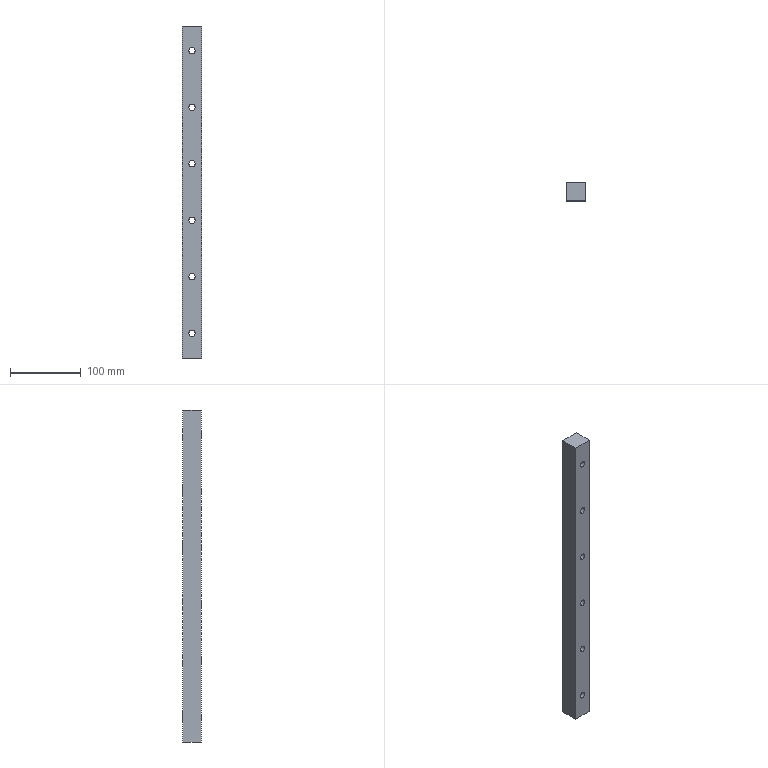Part | SolidWorks | features Extrusion 1, HoleWzd 1, LPattern 1 | 1 solid | 36 faces | box 28 x 26 x 470 mm | volume 326128 mm3 | cylinder 24 | plane 12 | commonest cylinder face diameters 9 x12 15 x12
STEP:
#1=CARTESIAN_POINT('',(0.,-13.,-439.5));
#2=VERTEX_POINT('',#1);
#3=CARTESIAN_POINT('',(0.,-13.,-430.5));
#4=VERTEX_POINT('',#3);
#5=CARTESIAN_POINT('',(0.,-13.,-435.));
#6=DIRECTION('',(0.,1.,0.));
#7=DIRECTION('',(0.,0.,1.));
#8=AXIS2_PLACEMENT_3D('',#5,#6,#7);
#9=CIRCLE('',#8,4.5);
#10=EDGE_CURVE('',#2,#4,#9,.T.);
#11=ORIENTED_EDGE('',*,*,#10,.F.);
#12=CARTESIAN_POINT('',(0.,4.,-439.5));
#13=VERTEX_POINT('',#12);
#14=CARTESIAN_POINT('',(0.,13.,-439.5));
#15=DIRECTION('',(0.,1.,0.));
#16=VECTOR('',#15,1000.);
#17=LINE('',#14,#16);
#18=EDGE_CURVE('',#2,#13,#17,.T.);
#19=ORIENTED_EDGE('',*,*,#18,.T.);
#20=CARTESIAN_POINT('',(0.,4.,-430.5));
#21=VERTEX_POINT('',#20);
#22=CARTESIAN_POINT('',(0.,4.,-435.));
#23=DIRECTION('',(0.,1.,0.));
#24=DIRECTION('',(0.,0.,1.));
#25=AXIS2_PLACEMENT_3D('',#22,#23,#24);
#26=CIRCLE('',#25,4.5);
#27=EDGE_CURVE('',#13,#21,#26,.T.);
#28=ORIENTED_EDGE('',*,*,#27,.T.);
#29=CARTESIAN_POINT('',(0.,13.,-430.5));
#30=DIRECTION('',(0.,1.,0.));
#31=VECTOR('',#30,1000.);
#32=LINE('',#29,#31);
#33=EDGE_CURVE('',#4,#21,#32,.T.);
#34=ORIENTED_EDGE('',*,*,#33,.F.);
#35=EDGE_LOOP('',(#11,#19,#28,#34));
#36=FACE_OUTER_BOUND('',#35,.T.);
#37=CARTESIAN_POINT('',(0.,13.,-435.));
#38=DIRECTION('',(0.,1.,0.));
#39=DIRECTION('',(0.,0.,1.));
#40=AXIS2_PLACEMENT_3D('',#37,#38,#39);
#41=CYLINDRICAL_SURFACE('',#40,4.5);
#42=ADVANCED_FACE('',(#36),#41,.F.);
#43=CARTESIAN_POINT('',(0.,4.,-442.5));
#44=VERTEX_POINT('',#43);
#45=CARTESIAN_POINT('',(0.,4.,-427.5));
#46=VERTEX_POINT('',#45);
#47=CARTESIAN_POINT('',(0.,4.,-435.));
#48=DIRECTION('',(0.,1.,0.));
#49=DIRECTION('',(0.,0.,1.));
#50=AXIS2_PLACEMENT_3D('',#47,#48,#49);
#51=CIRCLE('',#50,7.5);
#52=EDGE_CURVE('',#44,#46,#51,.T.);
#53=ORIENTED_EDGE('',*,*,#52,.F.);
#54=CARTESIAN_POINT('',(0.,13.,-442.5));
#55=VERTEX_POINT('',#54);
#56=CARTESIAN_POINT('',(0.,13.,-442.5));
#57=DIRECTION('',(0.,1.,0.));
#58=VECTOR('',#57,1000.);
#59=LINE('',#56,#58);
#60=EDGE_CURVE('',#44,#55,#59,.T.);
#61=ORIENTED_EDGE('',*,*,#60,.T.);
#62=CARTESIAN_POINT('',(0.,13.,-427.5));
#63=VERTEX_POINT('',#62);
#64=CARTESIAN_POINT('',(0.,13.,-435.));
#65=DIRECTION('',(0.,1.,0.));
#66=DIRECTION('',(0.,0.,1.));
#67=AXIS2_PLACEMENT_3D('',#64,#65,#66);
#68=CIRCLE('',#67,7.5);
#69=EDGE_CURVE('',#55,#63,#68,.T.);
#70=ORIENTED_EDGE('',*,*,#69,.T.);
#71=CARTESIAN_POINT('',(0.,13.,-427.5));
#72=DIRECTION('',(0.,1.,0.));
#73=VECTOR('',#72,1000.);
#74=LINE('',#71,#73);
#75=EDGE_CURVE('',#46,#63,#74,.T.);
#76=ORIENTED_EDGE('',*,*,#75,.F.);
#77=EDGE_LOOP('',(#53,#61,#70,#76));
#78=FACE_OUTER_BOUND('',#77,.T.);
#79=CARTESIAN_POINT('',(0.,13.,-435.));
#80=DIRECTION('',(0.,1.,0.));
#81=DIRECTION('',(0.,0.,1.));
#82=AXIS2_PLACEMENT_3D('',#79,#80,#81);
#83=CYLINDRICAL_SURFACE('',#82,7.5);
#84=ADVANCED_FACE('',(#78),#83,.F.);
#85=CARTESIAN_POINT('',(0.,-13.,-359.5));
#86=VERTEX_POINT('',#85);
#87=CARTESIAN_POINT('',(0.,-13.,-350.5));
#88=VERTEX_POINT('',#87);
#89=CARTESIAN_POINT('',(0.,-13.,-355.));
#90=DIRECTION('',(0.,1.,0.));
#91=DIRECTION('',(0.,0.,1.));
#92=AXIS2_PLACEMENT_3D('',#89,#90,#91);
#93=CIRCLE('',#92,4.5);
#94=EDGE_CURVE('',#86,#88,#93,.T.);
#95=ORIENTED_EDGE('',*,*,#94,.F.);
#96=CARTESIAN_POINT('',(0.,4.,-359.5));
#97=VERTEX_POINT('',#96);
#98=CARTESIAN_POINT('',(0.,13.,-359.5));
#99=DIRECTION('',(0.,1.,0.));
#100=VECTOR('',#99,1000.);
#101=LINE('',#98,#100);
#102=EDGE_CURVE('',#86,#97,#101,.T.);
#103=ORIENTED_EDGE('',*,*,#102,.T.);
#104=CARTESIAN_POINT('',(0.,4.,-350.5));
#105=VERTEX_POINT('',#104);
#106=CARTESIAN_POINT('',(0.,4.,-355.));
#107=DIRECTION('',(0.,1.,0.));
#108=DIRECTION('',(0.,0.,1.));
#109=AXIS2_PLACEMENT_3D('',#106,#107,#108);
#110=CIRCLE('',#109,4.5);
#111=EDGE_CURVE('',#97,#105,#110,.T.);
#112=ORIENTED_EDGE('',*,*,#111,.T.);
#113=CARTESIAN_POINT('',(0.,13.,-350.5));
#114=DIRECTION('',(0.,1.,0.));
#115=VECTOR('',#114,1000.);
#116=LINE('',#113,#115);
#117=EDGE_CURVE('',#88,#105,#116,.T.);
#118=ORIENTED_EDGE('',*,*,#117,.F.);
#119=EDGE_LOOP('',(#95,#103,#112,#118));
#120=FACE_OUTER_BOUND('',#119,.T.);
#121=CARTESIAN_POINT('',(0.,13.,-355.));
#122=DIRECTION('',(0.,1.,0.));
#123=DIRECTION('',(0.,0.,1.));
#124=AXIS2_PLACEMENT_3D('',#121,#122,#123);
#125=CYLINDRICAL_SURFACE('',#124,4.5);
#126=ADVANCED_FACE('',(#120),#125,.F.);
#127=CARTESIAN_POINT('',(0.,4.,-362.5));
#128=VERTEX_POINT('',#127);
#129=CARTESIAN_POINT('',(0.,4.,-347.5));
#130=VERTEX_POINT('',#129);
#131=CARTESIAN_POINT('',(0.,4.,-355.));
#132=DIRECTION('',(0.,1.,0.));
#133=DIRECTION('',(0.,0.,1.));
#134=AXIS2_PLACEMENT_3D('',#131,#132,#133);
#135=CIRCLE('',#134,7.5);
#136=EDGE_CURVE('',#128,#130,#135,.T.);
#137=ORIENTED_EDGE('',*,*,#136,.F.);
#138=CARTESIAN_POINT('',(0.,13.,-362.5));
#139=VERTEX_POINT('',#138);
#140=CARTESIAN_POINT('',(0.,13.,-362.5));
#141=DIRECTION('',(0.,1.,0.));
#142=VECTOR('',#141,1000.);
#143=LINE('',#140,#142);
#144=EDGE_CURVE('',#128,#139,#143,.T.);
#145=ORIENTED_EDGE('',*,*,#144,.T.);
#146=CARTESIAN_POINT('',(0.,13.,-347.5));
#147=VERTEX_POINT('',#146);
#148=CARTESIAN_POINT('',(0.,13.,-355.));
#149=DIRECTION('',(0.,1.,0.));
#150=DIRECTION('',(0.,0.,1.));
#151=AXIS2_PLACEMENT_3D('',#148,#149,#150);
#152=CIRCLE('',#151,7.5);
#153=EDGE_CURVE('',#139,#147,#152,.T.);
#154=ORIENTED_EDGE('',*,*,#153,.T.);
#155=CARTESIAN_POINT('',(0.,13.,-347.5));
#156=DIRECTION('',(0.,1.,0.));
#157=VECTOR('',#156,1000.);
#158=LINE('',#155,#157);
#159=EDGE_CURVE('',#130,#147,#158,.T.);
#160=ORIENTED_EDGE('',*,*,#159,.F.);
#161=EDGE_LOOP('',(#137,#145,#154,#160));
#162=FACE_OUTER_BOUND('',#161,.T.);
#163=CARTESIAN_POINT('',(0.,13.,-355.));
#164=DIRECTION('',(0.,1.,0.));
#165=DIRECTION('',(0.,0.,1.));
#166=AXIS2_PLACEMENT_3D('',#163,#164,#165);
#167=CYLINDRICAL_SURFACE('',#166,7.5);
#168=ADVANCED_FACE('',(#162),#167,.F.);
#169=CARTESIAN_POINT('',(0.,-13.,-279.5));
#170=VERTEX_POINT('',#169);
#171=CARTESIAN_POINT('',(0.,-13.,-270.5));
#172=VERTEX_POINT('',#171);
#173=CARTESIAN_POINT('',(0.,-13.,-275.));
#174=DIRECTION('',(0.,1.,0.));
#175=DIRECTION('',(0.,0.,1.));
#176=AXIS2_PLACEMENT_3D('',#173,#174,#175);
#177=CIRCLE('',#176,4.5);
#178=EDGE_CURVE('',#170,#172,#177,.T.);
#179=ORIENTED_EDGE('',*,*,#178,.F.);
#180=CARTESIAN_POINT('',(0.,4.,-279.5));
#181=VERTEX_POINT('',#180);
#182=CARTESIAN_POINT('',(0.,13.,-279.5));
#183=DIRECTION('',(0.,1.,0.));
#184=VECTOR('',#183,1000.);
#185=LINE('',#182,#184);
#186=EDGE_CURVE('',#170,#181,#185,.T.);
#187=ORIENTED_EDGE('',*,*,#186,.T.);
#188=CARTESIAN_POINT('',(0.,4.,-270.5));
#189=VERTEX_POINT('',#188);
#190=CARTESIAN_POINT('',(0.,4.,-275.));
#191=DIRECTION('',(0.,1.,0.));
#192=DIRECTION('',(0.,0.,1.));
#193=AXIS2_PLACEMENT_3D('',#190,#191,#192);
#194=CIRCLE('',#193,4.5);
#195=EDGE_CURVE('',#181,#189,#194,.T.);
#196=ORIENTED_EDGE('',*,*,#195,.T.);
#197=CARTESIAN_POINT('',(0.,13.,-270.5));
#198=DIRECTION('',(0.,1.,0.));
#199=VECTOR('',#198,1000.);
#200=LINE('',#197,#199);
#201=EDGE_CURVE('',#172,#189,#200,.T.);
#202=ORIENTED_EDGE('',*,*,#201,.F.);
#203=EDGE_LOOP('',(#179,#187,#196,#202));
#204=FACE_OUTER_BOUND('',#203,.T.);
#205=CARTESIAN_POINT('',(0.,13.,-275.));
#206=DIRECTION('',(0.,1.,0.));
#207=DIRECTION('',(0.,0.,1.));
#208=AXIS2_PLACEMENT_3D('',#205,#206,#207);
#209=CYLINDRICAL_SURFACE('',#208,4.5);
#210=ADVANCED_FACE('',(#204),#209,.F.);
#211=CARTESIAN_POINT('',(0.,4.,-282.5));
#212=VERTEX_POINT('',#211);
#213=CARTESIAN_POINT('',(0.,4.,-267.5));
#214=VERTEX_POINT('',#213);
#215=CARTESIAN_POINT('',(0.,4.,-275.));
#216=DIRECTION('',(0.,1.,0.));
#217=DIRECTION('',(0.,0.,1.));
#218=AXIS2_PLACEMENT_3D('',#215,#216,#217);
#219=CIRCLE('',#218,7.5);
#220=EDGE_CURVE('',#212,#214,#219,.T.);
#221=ORIENTED_EDGE('',*,*,#220,.F.);
#222=CARTESIAN_POINT('',(0.,13.,-282.5));
#223=VERTEX_POINT('',#222);
#224=CARTESIAN_POINT('',(0.,13.,-282.5));
#225=DIRECTION('',(0.,1.,0.));
#226=VECTOR('',#225,1000.);
#227=LINE('',#224,#226);
#228=EDGE_CURVE('',#212,#223,#227,.T.);
#229=ORIENTED_EDGE('',*,*,#228,.T.);
#230=CARTESIAN_POINT('',(0.,13.,-267.5));
#231=VERTEX_POINT('',#230);
#232=CARTESIAN_POINT('',(0.,13.,-275.));
#233=DIRECTION('',(0.,1.,0.));
#234=DIRECTION('',(0.,0.,1.));
#235=AXIS2_PLACEMENT_3D('',#232,#233,#234);
#236=CIRCLE('',#235,7.5);
#237=EDGE_CURVE('',#223,#231,#236,.T.);
#238=ORIENTED_EDGE('',*,*,#237,.T.);
#239=CARTESIAN_POINT('',(0.,13.,-267.5));
#240=DIRECTION('',(0.,1.,0.));
#241=VECTOR('',#240,1000.);
#242=LINE('',#239,#241);
#243=EDGE_CURVE('',#214,#231,#242,.T.);
#244=ORIENTED_EDGE('',*,*,#243,.F.);
#245=EDGE_LOOP('',(#221,#229,#238,#244));
#246=FACE_OUTER_BOUND('',#245,.T.);
#247=CARTESIAN_POINT('',(0.,13.,-275.));
#248=DIRECTION('',(0.,1.,0.));
#249=DIRECTION('',(0.,0.,1.));
#250=AXIS2_PLACEMENT_3D('',#247,#248,#249);
#251=CYLINDRICAL_SURFACE('',#250,7.5);
#252=ADVANCED_FACE('',(#246),#251,.F.);
#253=CARTESIAN_POINT('',(0.,-13.,-199.5));
#254=VERTEX_POINT('',#253);
#255=CARTESIAN_POINT('',(0.,-13.,-190.5));
#256=VERTEX_POINT('',#255);
#257=CARTESIAN_POINT('',(0.,-13.,-195.));
#258=DIRECTION('',(0.,1.,0.));
#259=DIRECTION('',(0.,0.,1.));
#260=AXIS2_PLACEMENT_3D('',#257,#258,#259);
#261=CIRCLE('',#260,4.5);
#262=EDGE_CURVE('',#254,#256,#261,.T.);
#263=ORIENTED_EDGE('',*,*,#262,.F.);
#264=CARTESIAN_POINT('',(0.,4.,-199.5));
#265=VERTEX_POINT('',#264);
#266=CARTESIAN_POINT('',(0.,13.,-199.5));
#267=DIRECTION('',(0.,1.,0.));
#268=VECTOR('',#267,1000.);
#269=LINE('',#266,#268);
#270=EDGE_CURVE('',#254,#265,#269,.T.);
#271=ORIENTED_EDGE('',*,*,#270,.T.);
#272=CARTESIAN_POINT('',(0.,4.,-190.5));
#273=VERTEX_POINT('',#272);
#274=CARTESIAN_POINT('',(0.,4.,-195.));
#275=DIRECTION('',(0.,1.,0.));
#276=DIRECTION('',(0.,0.,1.));
#277=AXIS2_PLACEMENT_3D('',#274,#275,#276);
#278=CIRCLE('',#277,4.5);
#279=EDGE_CURVE('',#265,#273,#278,.T.);
#280=ORIENTED_EDGE('',*,*,#279,.T.);
#281=CARTESIAN_POINT('',(0.,13.,-190.5));
#282=DIRECTION('',(0.,1.,0.));
#283=VECTOR('',#282,1000.);
#284=LINE('',#281,#283);
#285=EDGE_CURVE('',#256,#273,#284,.T.);
#286=ORIENTED_EDGE('',*,*,#285,.F.);
#287=EDGE_LOOP('',(#263,#271,#280,#286));
#288=FACE_OUTER_BOUND('',#287,.T.);
#289=CARTESIAN_POINT('',(0.,13.,-195.));
#290=DIRECTION('',(0.,1.,0.));
#291=DIRECTION('',(0.,0.,1.));
#292=AXIS2_PLACEMENT_3D('',#289,#290,#291);
#293=CYLINDRICAL_SURFACE('',#292,4.5);
#294=ADVANCED_FACE('',(#288),#293,.F.);
#295=CARTESIAN_POINT('',(0.,4.,-202.5));
#296=VERTEX_POINT('',#295);
#297=CARTESIAN_POINT('',(0.,4.,-187.5));
#298=VERTEX_POINT('',#297);
#299=CARTESIAN_POINT('',(0.,4.,-195.));
#300=DIRECTION('',(0.,1.,0.));
#301=DIRECTION('',(0.,0.,1.));
#302=AXIS2_PLACEMENT_3D('',#299,#300,#301);
#303=CIRCLE('',#302,7.5);
#304=EDGE_CURVE('',#296,#298,#303,.T.);
#305=ORIENTED_EDGE('',*,*,#304,.F.);
#306=CARTESIAN_POINT('',(0.,13.,-202.5));
#307=VERTEX_POINT('',#306);
#308=CARTESIAN_POINT('',(0.,13.,-202.5));
#309=DIRECTION('',(0.,1.,0.));
#310=VECTOR('',#309,1000.);
#311=LINE('',#308,#310);
#312=EDGE_CURVE('',#296,#307,#311,.T.);
#313=ORIENTED_EDGE('',*,*,#312,.T.);
#314=CARTESIAN_POINT('',(0.,13.,-187.5));
#315=VERTEX_POINT('',#314);
#316=CARTESIAN_POINT('',(0.,13.,-195.));
#317=DIRECTION('',(0.,1.,0.));
#318=DIRECTION('',(0.,0.,1.));
#319=AXIS2_PLACEMENT_3D('',#316,#317,#318);
#320=CIRCLE('',#319,7.5);
#321=EDGE_CURVE('',#307,#315,#320,.T.);
#322=ORIENTED_EDGE('',*,*,#321,.T.);
#323=CARTESIAN_POINT('',(0.,13.,-187.5));
#324=DIRECTION('',(0.,1.,0.));
#325=VECTOR('',#324,1000.);
#326=LINE('',#323,#325);
#327=EDGE_CURVE('',#298,#315,#326,.T.);
#328=ORIENTED_EDGE('',*,*,#327,.F.);
#329=EDGE_LOOP('',(#305,#313,#322,#328));
#330=FACE_OUTER_BOUND('',#329,.T.);
#331=CARTESIAN_POINT('',(0.,13.,-195.));
#332=DIRECTION('',(0.,1.,0.));
#333=DIRECTION('',(0.,0.,1.));
#334=AXIS2_PLACEMENT_3D('',#331,#332,#333);
#335=CYLINDRICAL_SURFACE('',#334,7.5);
#336=ADVANCED_FACE('',(#330),#335,.F.);
#337=CARTESIAN_POINT('',(0.,4.,-122.5));
#338=VERTEX_POINT('',#337);
#339=CARTESIAN_POINT('',(0.,4.,-107.5));
#340=VERTEX_POINT('',#339);
#341=CARTESIAN_POINT('',(0.,4.,-115.));
#342=DIRECTION('',(0.,1.,0.));
#343=DIRECTION('',(0.,0.,1.));
#344=AXIS2_PLACEMENT_3D('',#341,#342,#343);
#345=CIRCLE('',#344,7.5);
#346=EDGE_CURVE('',#338,#340,#345,.T.);
#347=ORIENTED_EDGE('',*,*,#346,.F.);
#348=CARTESIAN_POINT('',(0.,13.,-122.5));
#349=VERTEX_POINT('',#348);
#350=CARTESIAN_POINT('',(0.,13.,-122.5));
#351=DIRECTION('',(0.,1.,0.));
#352=VECTOR('',#351,1000.);
#353=LINE('',#350,#352);
#354=EDGE_CURVE('',#338,#349,#353,.T.);
#355=ORIENTED_EDGE('',*,*,#354,.T.);
#356=CARTESIAN_POINT('',(0.,13.,-107.5));
#357=VERTEX_POINT('',#356);
#358=CARTESIAN_POINT('',(0.,13.,-115.));
#359=DIRECTION('',(0.,1.,0.));
#360=DIRECTION('',(0.,0.,1.));
#361=AXIS2_PLACEMENT_3D('',#358,#359,#360);
#362=CIRCLE('',#361,7.5);
#363=EDGE_CURVE('',#349,#357,#362,.T.);
#364=ORIENTED_EDGE('',*,*,#363,.T.);
#365=CARTESIAN_POINT('',(0.,13.,-107.5));
#366=DIRECTION('',(0.,1.,0.));
#367=VECTOR('',#366,1000.);
#368=LINE('',#365,#367);
#369=EDGE_CURVE('',#340,#357,#368,.T.);
#370=ORIENTED_EDGE('',*,*,#369,.F.);
#371=EDGE_LOOP('',(#347,#355,#364,#370));
#372=FACE_OUTER_BOUND('',#371,.T.);
#373=CARTESIAN_POINT('',(0.,13.,-115.));
#374=DIRECTION('',(0.,1.,0.));
#375=DIRECTION('',(0.,0.,1.));
#376=AXIS2_PLACEMENT_3D('',#373,#374,#375);
#377=CYLINDRICAL_SURFACE('',#376,7.5);
#378=ADVANCED_FACE('',(#372),#377,.F.);
#379=CARTESIAN_POINT('',(0.,-13.,-119.5));
#380=VERTEX_POINT('',#379);
#381=CARTESIAN_POINT('',(0.,-13.,-110.5));
#382=VERTEX_POINT('',#381);
#383=CARTESIAN_POINT('',(0.,-13.,-115.));
#384=DIRECTION('',(0.,1.,0.));
#385=DIRECTION('',(0.,0.,1.));
#386=AXIS2_PLACEMENT_3D('',#383,#384,#385);
#387=CIRCLE('',#386,4.5);
#388=EDGE_CURVE('',#380,#382,#387,.T.);
#389=ORIENTED_EDGE('',*,*,#388,.F.);
#390=CARTESIAN_POINT('',(0.,4.,-119.5));
#391=VERTEX_POINT('',#390);
#392=CARTESIAN_POINT('',(0.,13.,-119.5));
#393=DIRECTION('',(0.,1.,0.));
#394=VECTOR('',#393,1000.);
#395=LINE('',#392,#394);
#396=EDGE_CURVE('',#380,#391,#395,.T.);
#397=ORIENTED_EDGE('',*,*,#396,.T.);
#398=CARTESIAN_POINT('',(0.,4.,-110.5));
#399=VERTEX_POINT('',#398);
#400=CARTESIAN_POINT('',(0.,4.,-115.));
#401=DIRECTION('',(0.,1.,0.));
#402=DIRECTION('',(0.,0.,1.));
#403=AXIS2_PLACEMENT_3D('',#400,#401,#402);
#404=CIRCLE('',#403,4.5);
#405=EDGE_CURVE('',#391,#399,#404,.T.);
#406=ORIENTED_EDGE('',*,*,#405,.T.);
#407=CARTESIAN_POINT('',(0.,13.,-110.5));
#408=DIRECTION('',(0.,1.,0.));
#409=VECTOR('',#408,1000.);
#410=LINE('',#407,#409);
#411=EDGE_CURVE('',#382,#399,#410,.T.);
#412=ORIENTED_EDGE('',*,*,#411,.F.);
#413=EDGE_LOOP('',(#389,#397,#406,#412));
#414=FACE_OUTER_BOUND('',#413,.T.);
#415=CARTESIAN_POINT('',(0.,13.,-115.));
#416=DIRECTION('',(0.,1.,0.));
#417=DIRECTION('',(0.,0.,1.));
#418=AXIS2_PLACEMENT_3D('',#415,#416,#417);
#419=CYLINDRICAL_SURFACE('',#418,4.5);
#420=ADVANCED_FACE('',(#414),#419,.F.);
#421=CARTESIAN_POINT('',(0.,4.,-42.5));
#422=VERTEX_POINT('',#421);
#423=CARTESIAN_POINT('',(0.,4.,-27.5));
#424=VERTEX_POINT('',#423);
#425=CARTESIAN_POINT('',(0.,4.,-35.));
#426=DIRECTION('',(0.,1.,0.));
#427=DIRECTION('',(0.,0.,1.));
#428=AXIS2_PLACEMENT_3D('',#425,#426,#427);
#429=CIRCLE('',#428,7.5);
#430=EDGE_CURVE('',#422,#424,#429,.T.);
#431=ORIENTED_EDGE('',*,*,#430,.F.);
#432=CARTESIAN_POINT('',(0.,13.,-42.5));
#433=VERTEX_POINT('',#432);
#434=CARTESIAN_POINT('',(0.,13.,-42.5));
#435=DIRECTION('',(0.,1.,0.));
#436=VECTOR('',#435,1000.);
#437=LINE('',#434,#436);
#438=EDGE_CURVE('',#422,#433,#437,.T.);
#439=ORIENTED_EDGE('',*,*,#438,.T.);
#440=CARTESIAN_POINT('',(0.,13.,-27.5));
#441=VERTEX_POINT('',#440);
#442=CARTESIAN_POINT('',(0.,13.,-35.));
#443=DIRECTION('',(0.,1.,0.));
#444=DIRECTION('',(0.,0.,1.));
#445=AXIS2_PLACEMENT_3D('',#442,#443,#444);
#446=CIRCLE('',#445,7.5);
#447=EDGE_CURVE('',#433,#441,#446,.T.);
#448=ORIENTED_EDGE('',*,*,#447,.T.);
#449=CARTESIAN_POINT('',(0.,13.,-27.5));
#450=DIRECTION('',(0.,1.,0.));
#451=VECTOR('',#450,1000.);
#452=LINE('',#449,#451);
#453=EDGE_CURVE('',#424,#441,#452,.T.);
#454=ORIENTED_EDGE('',*,*,#453,.F.);
#455=EDGE_LOOP('',(#431,#439,#448,#454));
#456=FACE_OUTER_BOUND('',#455,.T.);
#457=CARTESIAN_POINT('',(0.,13.,-35.));
#458=DIRECTION('',(0.,1.,0.));
#459=DIRECTION('',(0.,0.,1.));
#460=AXIS2_PLACEMENT_3D('',#457,#458,#459);
#461=CYLINDRICAL_SURFACE('',#460,7.5);
#462=ADVANCED_FACE('',(#456),#461,.F.);
#463=CARTESIAN_POINT('',(0.,-13.,-39.5));
#464=VERTEX_POINT('',#463);
#465=CARTESIAN_POINT('',(0.,-13.,-30.5));
#466=VERTEX_POINT('',#465);
#467=CARTESIAN_POINT('',(0.,-13.,-35.));
#468=DIRECTION('',(0.,1.,0.));
#469=DIRECTION('',(0.,0.,1.));
#470=AXIS2_PLACEMENT_3D('',#467,#468,#469);
#471=CIRCLE('',#470,4.5);
#472=EDGE_CURVE('',#464,#466,#471,.T.);
#473=ORIENTED_EDGE('',*,*,#472,.F.);
#474=CARTESIAN_POINT('',(0.,4.,-39.5));
#475=VERTEX_POINT('',#474);
#476=CARTESIAN_POINT('',(0.,13.,-39.5));
#477=DIRECTION('',(0.,1.,0.));
#478=VECTOR('',#477,1000.);
#479=LINE('',#476,#478);
#480=EDGE_CURVE('',#464,#475,#479,.T.);
#481=ORIENTED_EDGE('',*,*,#480,.T.);
#482=CARTESIAN_POINT('',(0.,4.,-30.5));
#483=VERTEX_POINT('',#482);
#484=CARTESIAN_POINT('',(0.,4.,-35.));
#485=DIRECTION('',(0.,1.,0.));
#486=DIRECTION('',(0.,0.,1.));
#487=AXIS2_PLACEMENT_3D('',#484,#485,#486);
#488=CIRCLE('',#487,4.5);
#489=EDGE_CURVE('',#475,#483,#488,.T.);
#490=ORIENTED_EDGE('',*,*,#489,.T.);
#491=CARTESIAN_POINT('',(0.,13.,-30.5));
#492=DIRECTION('',(0.,1.,0.));
#493=VECTOR('',#492,1000.);
#494=LINE('',#491,#493);
#495=EDGE_CURVE('',#466,#483,#494,.T.);
#496=ORIENTED_EDGE('',*,*,#495,.F.);
#497=EDGE_LOOP('',(#473,#481,#490,#496));
#498=FACE_OUTER_BOUND('',#497,.T.);
#499=CARTESIAN_POINT('',(0.,13.,-35.));
#500=DIRECTION('',(0.,1.,0.));
#501=DIRECTION('',(0.,0.,1.));
#502=AXIS2_PLACEMENT_3D('',#499,#500,#501);
#503=CYLINDRICAL_SURFACE('',#502,4.5);
#504=ADVANCED_FACE('',(#498),#503,.F.);
#505=CARTESIAN_POINT('',(14.,-13.,0.));
#506=VERTEX_POINT('',#505);
#507=CARTESIAN_POINT('',(14.,13.,0.));
#508=VERTEX_POINT('',#507);
#509=CARTESIAN_POINT('',(14.,13.,0.));
#510=DIRECTION('',(0.,1.,0.));
#511=VECTOR('',#510,1000.);
#512=LINE('',#509,#511);
#513=EDGE_CURVE('',#506,#508,#512,.T.);
#514=ORIENTED_EDGE('',*,*,#513,.F.);
#515=CARTESIAN_POINT('',(14.,-13.,-470.));
#516=VERTEX_POINT('',#515);
#517=CARTESIAN_POINT('',(14.,-13.,-470.));
#518=DIRECTION('',(0.,0.,1.));
#519=VECTOR('',#518,1000.);
#520=LINE('',#517,#519);
#521=EDGE_CURVE('',#516,#506,#520,.T.);
#522=ORIENTED_EDGE('',*,*,#521,.F.);
#523=CARTESIAN_POINT('',(14.,13.,-470.));
#524=VERTEX_POINT('',#523);
#525=CARTESIAN_POINT('',(14.,13.,-470.));
#526=DIRECTION('',(0.,1.,0.));
#527=VECTOR('',#526,1000.);
#528=LINE('',#525,#527);
#529=EDGE_CURVE('',#516,#524,#528,.T.);
#530=ORIENTED_EDGE('',*,*,#529,.T.);
#531=CARTESIAN_POINT('',(14.,13.,-470.));
#532=DIRECTION('',(0.,0.,1.));
#533=VECTOR('',#532,1000.);
#534=LINE('',#531,#533);
#535=EDGE_CURVE('',#524,#508,#534,.T.);
#536=ORIENTED_EDGE('',*,*,#535,.T.);
#537=EDGE_LOOP('',(#514,#522,#530,#536));
#538=FACE_OUTER_BOUND('',#537,.T.);
#539=CARTESIAN_POINT('',(14.,13.,-470.));
#540=DIRECTION('',(1.,0.,0.));
#541=DIRECTION('',(0.,1.,0.));
#542=AXIS2_PLACEMENT_3D('',#539,#540,#541);
#543=PLANE('',#542);
#544=ADVANCED_FACE('',(#538),#543,.T.);
#545=CARTESIAN_POINT('',(0.,-13.,-115.));
#546=DIRECTION('',(0.,1.,0.));
#547=DIRECTION('',(0.,0.,1.));
#548=AXIS2_PLACEMENT_3D('',#545,#546,#547);
#549=CIRCLE('',#548,4.5);
#550=EDGE_CURVE('',#382,#380,#549,.T.);
#551=ORIENTED_EDGE('',*,*,#550,.T.);
#552=ORIENTED_EDGE('',*,*,#388,.T.);
#553=EDGE_LOOP('',(#551,#552));
#554=FACE_BOUND('',#553,.T.);
#555=CARTESIAN_POINT('',(0.,-13.,-35.));
#556=DIRECTION('',(0.,1.,0.));
#557=DIRECTION('',(0.,0.,1.));
#558=AXIS2_PLACEMENT_3D('',#555,#556,#557);
#559=CIRCLE('',#558,4.5);
#560=EDGE_CURVE('',#466,#464,#559,.T.);
#561=ORIENTED_EDGE('',*,*,#560,.T.);
#562=ORIENTED_EDGE('',*,*,#472,.T.);
#563=EDGE_LOOP('',(#561,#562));
#564=FACE_BOUND('',#563,.T.);
#565=CARTESIAN_POINT('',(-14.,-13.,0.));
#566=VERTEX_POINT('',#565);
#567=CARTESIAN_POINT('',(-14.,-13.,0.));
#568=DIRECTION('',(1.,0.,0.));
#569=VECTOR('',#568,1000.);
#570=LINE('',#567,#569);
#571=EDGE_CURVE('',#566,#506,#570,.T.);
#572=ORIENTED_EDGE('',*,*,#571,.F.);
#573=CARTESIAN_POINT('',(-14.,-13.,-470.));
#574=VERTEX_POINT('',#573);
#575=CARTESIAN_POINT('',(-14.,-13.,-470.));
#576=DIRECTION('',(0.,0.,1.));
#577=VECTOR('',#576,1000.);
#578=LINE('',#575,#577);
#579=EDGE_CURVE('',#574,#566,#578,.T.);
#580=ORIENTED_EDGE('',*,*,#579,.F.);
#581=CARTESIAN_POINT('',(-14.,-13.,-470.));
#582=DIRECTION('',(1.,0.,0.));
#583=VECTOR('',#582,1000.);
#584=LINE('',#581,#583);
#585=EDGE_CURVE('',#574,#516,#584,.T.);
#586=ORIENTED_EDGE('',*,*,#585,.T.);
#587=ORIENTED_EDGE('',*,*,#521,.T.);
#588=EDGE_LOOP('',(#572,#580,#586,#587));
#589=FACE_OUTER_BOUND('',#588,.T.);
#590=CARTESIAN_POINT('',(0.,-13.,-195.));
#591=DIRECTION('',(0.,1.,0.));
#592=DIRECTION('',(0.,0.,1.));
#593=AXIS2_PLACEMENT_3D('',#590,#591,#592);
#594=CIRCLE('',#593,4.5);
#595=EDGE_CURVE('',#256,#254,#594,.T.);
#596=ORIENTED_EDGE('',*,*,#595,.T.);
#597=ORIENTED_EDGE('',*,*,#262,.T.);
#598=EDGE_LOOP('',(#596,#597));
#599=FACE_BOUND('',#598,.T.);
#600=CARTESIAN_POINT('',(0.,-13.,-275.));
#601=DIRECTION('',(0.,1.,0.));
#602=DIRECTION('',(0.,0.,1.));
#603=AXIS2_PLACEMENT_3D('',#600,#601,#602);
#604=CIRCLE('',#603,4.5);
#605=EDGE_CURVE('',#172,#170,#604,.T.);
#606=ORIENTED_EDGE('',*,*,#605,.T.);
#607=ORIENTED_EDGE('',*,*,#178,.T.);
#608=EDGE_LOOP('',(#606,#607));
#609=FACE_BOUND('',#608,.T.);
#610=CARTESIAN_POINT('',(0.,-13.,-355.));
#611=DIRECTION('',(0.,1.,0.));
#612=DIRECTION('',(0.,0.,1.));
#613=AXIS2_PLACEMENT_3D('',#610,#611,#612);
#614=CIRCLE('',#613,4.5);
#615=EDGE_CURVE('',#88,#86,#614,.T.);
#616=ORIENTED_EDGE('',*,*,#615,.T.);
#617=ORIENTED_EDGE('',*,*,#94,.T.);
#618=EDGE_LOOP('',(#616,#617));
#619=FACE_BOUND('',#618,.T.);
#620=CARTESIAN_POINT('',(0.,-13.,-435.));
#621=DIRECTION('',(0.,1.,0.));
#622=DIRECTION('',(0.,0.,1.));
#623=AXIS2_PLACEMENT_3D('',#620,#621,#622);
#624=CIRCLE('',#623,4.5);
#625=EDGE_CURVE('',#4,#2,#624,.T.);
#626=ORIENTED_EDGE('',*,*,#625,.T.);
#627=ORIENTED_EDGE('',*,*,#10,.T.);
#628=EDGE_LOOP('',(#626,#627));
#629=FACE_BOUND('',#628,.T.);
#630=CARTESIAN_POINT('',(-14.,-13.,-470.));
#631=DIRECTION('',(0.,-1.,0.));
#632=DIRECTION('',(0.,0.,-1.));
#633=AXIS2_PLACEMENT_3D('',#630,#631,#632);
#634=PLANE('',#633);
#635=ADVANCED_FACE('',(#554,#564,#589,#599,#609,#619,#629),#634,.T.);
#636=CARTESIAN_POINT('',(-14.,13.,0.));
#637=VERTEX_POINT('',#636);
#638=CARTESIAN_POINT('',(-14.,13.,0.));
#639=DIRECTION('',(0.,-1.,0.));
#640=VECTOR('',#639,1000.);
#641=LINE('',#638,#640);
#642=EDGE_CURVE('',#637,#566,#641,.T.);
#643=ORIENTED_EDGE('',*,*,#642,.F.);
#644=CARTESIAN_POINT('',(-14.,13.,-470.));
#645=VERTEX_POINT('',#644);
#646=CARTESIAN_POINT('',(-14.,13.,-470.));
#647=DIRECTION('',(0.,0.,1.));
#648=VECTOR('',#647,1000.);
#649=LINE('',#646,#648);
#650=EDGE_CURVE('',#645,#637,#649,.T.);
#651=ORIENTED_EDGE('',*,*,#650,.F.);
#652=CARTESIAN_POINT('',(-14.,13.,-470.));
#653=DIRECTION('',(0.,-1.,0.));
#654=VECTOR('',#653,1000.);
#655=LINE('',#652,#654);
#656=EDGE_CURVE('',#645,#574,#655,.T.);
#657=ORIENTED_EDGE('',*,*,#656,.T.);
#658=ORIENTED_EDGE('',*,*,#579,.T.);
#659=EDGE_LOOP('',(#643,#651,#657,#658));
#660=FACE_OUTER_BOUND('',#659,.T.);
#661=CARTESIAN_POINT('',(-14.,13.,-470.));
#662=DIRECTION('',(-1.,0.,0.));
#663=DIRECTION('',(0.,-1.,0.));
#664=AXIS2_PLACEMENT_3D('',#661,#662,#663);
#665=PLANE('',#664);
#666=ADVANCED_FACE('',(#660),#665,.T.);
#667=CARTESIAN_POINT('',(0.,13.,-115.));
#668=DIRECTION('',(0.,1.,0.));
#669=DIRECTION('',(0.,0.,1.));
#670=AXIS2_PLACEMENT_3D('',#667,#668,#669);
#671=CIRCLE('',#670,7.5);
#672=EDGE_CURVE('',#357,#349,#671,.T.);
#673=ORIENTED_EDGE('',*,*,#672,.F.);
#674=ORIENTED_EDGE('',*,*,#363,.F.);
#675=EDGE_LOOP('',(#673,#674));
#676=FACE_BOUND('',#675,.T.);
#677=CARTESIAN_POINT('',(0.,13.,-35.));
#678=DIRECTION('',(0.,1.,0.));
#679=DIRECTION('',(0.,0.,1.));
#680=AXIS2_PLACEMENT_3D('',#677,#678,#679);
#681=CIRCLE('',#680,7.5);
#682=EDGE_CURVE('',#441,#433,#681,.T.);
#683=ORIENTED_EDGE('',*,*,#682,.F.);
#684=ORIENTED_EDGE('',*,*,#447,.F.);
#685=EDGE_LOOP('',(#683,#684));
#686=FACE_BOUND('',#685,.T.);
#687=CARTESIAN_POINT('',(-14.,13.,0.));
#688=DIRECTION('',(-1.,0.,0.));
#689=VECTOR('',#688,1000.);
#690=LINE('',#687,#689);
#691=EDGE_CURVE('',#508,#637,#690,.T.);
#692=ORIENTED_EDGE('',*,*,#691,.F.);
#693=ORIENTED_EDGE('',*,*,#535,.F.);
#694=CARTESIAN_POINT('',(-14.,13.,-470.));
#695=DIRECTION('',(-1.,0.,0.));
#696=VECTOR('',#695,1000.);
#697=LINE('',#694,#696);
#698=EDGE_CURVE('',#524,#645,#697,.T.);
#699=ORIENTED_EDGE('',*,*,#698,.T.);
#700=ORIENTED_EDGE('',*,*,#650,.T.);
#701=EDGE_LOOP('',(#692,#693,#699,#700));
#702=FACE_OUTER_BOUND('',#701,.T.);
#703=CARTESIAN_POINT('',(0.,13.,-195.));
#704=DIRECTION('',(0.,1.,0.));
#705=DIRECTION('',(0.,0.,1.));
#706=AXIS2_PLACEMENT_3D('',#703,#704,#705);
#707=CIRCLE('',#706,7.5);
#708=EDGE_CURVE('',#315,#307,#707,.T.);
#709=ORIENTED_EDGE('',*,*,#708,.F.);
#710=ORIENTED_EDGE('',*,*,#321,.F.);
#711=EDGE_LOOP('',(#709,#710));
#712=FACE_BOUND('',#711,.T.);
#713=CARTESIAN_POINT('',(0.,13.,-275.));
#714=DIRECTION('',(0.,1.,0.));
#715=DIRECTION('',(0.,0.,1.));
#716=AXIS2_PLACEMENT_3D('',#713,#714,#715);
#717=CIRCLE('',#716,7.5);
#718=EDGE_CURVE('',#231,#223,#717,.T.);
#719=ORIENTED_EDGE('',*,*,#718,.F.);
#720=ORIENTED_EDGE('',*,*,#237,.F.);
#721=EDGE_LOOP('',(#719,#720));
#722=FACE_BOUND('',#721,.T.);
#723=CARTESIAN_POINT('',(0.,13.,-355.));
#724=DIRECTION('',(0.,1.,0.));
#725=DIRECTION('',(0.,0.,1.));
#726=AXIS2_PLACEMENT_3D('',#723,#724,#725);
#727=CIRCLE('',#726,7.5);
#728=EDGE_CURVE('',#147,#139,#727,.T.);
#729=ORIENTED_EDGE('',*,*,#728,.F.);
#730=ORIENTED_EDGE('',*,*,#153,.F.);
#731=EDGE_LOOP('',(#729,#730));
#732=FACE_BOUND('',#731,.T.);
#733=CARTESIAN_POINT('',(0.,13.,-435.));
#734=DIRECTION('',(0.,1.,0.));
#735=DIRECTION('',(0.,0.,1.));
#736=AXIS2_PLACEMENT_3D('',#733,#734,#735);
#737=CIRCLE('',#736,7.5);
#738=EDGE_CURVE('',#63,#55,#737,.T.);
#739=ORIENTED_EDGE('',*,*,#738,.F.);
#740=ORIENTED_EDGE('',*,*,#69,.F.);
#741=EDGE_LOOP('',(#739,#740));
#742=FACE_BOUND('',#741,.T.);
#743=CARTESIAN_POINT('',(-14.,13.,-470.));
#744=DIRECTION('',(0.,1.,0.));
#745=DIRECTION('',(0.,0.,1.));
#746=AXIS2_PLACEMENT_3D('',#743,#744,#745);
#747=PLANE('',#746);
#748=ADVANCED_FACE('',(#676,#686,#702,#712,#722,#732,#742),#747,.T.);
#749=ORIENTED_EDGE('',*,*,#529,.F.);
#750=ORIENTED_EDGE('',*,*,#585,.F.);
#751=ORIENTED_EDGE('',*,*,#656,.F.);
#752=ORIENTED_EDGE('',*,*,#698,.F.);
#753=EDGE_LOOP('',(#749,#750,#751,#752));
#754=FACE_OUTER_BOUND('',#753,.T.);
#755=CARTESIAN_POINT('',(14.,-13.,-470.));
#756=DIRECTION('',(0.,0.,1.));
#757=DIRECTION('',(1.,0.,0.));
#758=AXIS2_PLACEMENT_3D('',#755,#756,#757);
#759=PLANE('',#758);
#760=ADVANCED_FACE('',(#754),#759,.F.);
#761=ORIENTED_EDGE('',*,*,#513,.T.);
#762=ORIENTED_EDGE('',*,*,#691,.T.);
#763=ORIENTED_EDGE('',*,*,#642,.T.);
#764=ORIENTED_EDGE('',*,*,#571,.T.);
#765=EDGE_LOOP('',(#761,#762,#763,#764));
#766=FACE_OUTER_BOUND('',#765,.T.);
#767=CARTESIAN_POINT('',(14.,-13.,0.));
#768=DIRECTION('',(0.,0.,1.));
#769=DIRECTION('',(1.,0.,0.));
#770=AXIS2_PLACEMENT_3D('',#767,#768,#769);
#771=PLANE('',#770);
#772=ADVANCED_FACE('',(#766),#771,.T.);
#773=ORIENTED_EDGE('',*,*,#480,.F.);
#774=ORIENTED_EDGE('',*,*,#560,.F.);
#775=ORIENTED_EDGE('',*,*,#495,.T.);
#776=CARTESIAN_POINT('',(0.,4.,-35.));
#777=DIRECTION('',(0.,1.,0.));
#778=DIRECTION('',(0.,0.,1.));
#779=AXIS2_PLACEMENT_3D('',#776,#777,#778);
#780=CIRCLE('',#779,4.5);
#781=EDGE_CURVE('',#483,#475,#780,.T.);
#782=ORIENTED_EDGE('',*,*,#781,.T.);
#783=EDGE_LOOP('',(#773,#774,#775,#782));
#784=FACE_OUTER_BOUND('',#783,.T.);
#785=CARTESIAN_POINT('',(0.,13.,-35.));
#786=DIRECTION('',(0.,1.,0.));
#787=DIRECTION('',(0.,0.,1.));
#788=AXIS2_PLACEMENT_3D('',#785,#786,#787);
#789=CYLINDRICAL_SURFACE('',#788,4.5);
#790=ADVANCED_FACE('',(#784),#789,.F.);
#791=ORIENTED_EDGE('',*,*,#781,.F.);
#792=ORIENTED_EDGE('',*,*,#489,.F.);
#793=EDGE_LOOP('',(#791,#792));
#794=FACE_BOUND('',#793,.T.);
#795=CARTESIAN_POINT('',(0.,4.,-35.));
#796=DIRECTION('',(0.,1.,0.));
#797=DIRECTION('',(0.,0.,1.));
#798=AXIS2_PLACEMENT_3D('',#795,#796,#797);
#799=CIRCLE('',#798,7.5);
#800=EDGE_CURVE('',#424,#422,#799,.T.);
#801=ORIENTED_EDGE('',*,*,#800,.T.);
#802=ORIENTED_EDGE('',*,*,#430,.T.);
#803=EDGE_LOOP('',(#801,#802));
#804=FACE_OUTER_BOUND('',#803,.T.);
#805=CARTESIAN_POINT('',(4.5,4.,-35.));
#806=DIRECTION('',(0.,-1.,0.));
#807=DIRECTION('',(0.,0.,-1.));
#808=AXIS2_PLACEMENT_3D('',#805,#806,#807);
#809=PLANE('',#808);
#810=ADVANCED_FACE('',(#794,#804),#809,.F.);
#811=ORIENTED_EDGE('',*,*,#438,.F.);
#812=ORIENTED_EDGE('',*,*,#800,.F.);
#813=ORIENTED_EDGE('',*,*,#453,.T.);
#814=ORIENTED_EDGE('',*,*,#682,.T.);
#815=EDGE_LOOP('',(#811,#812,#813,#814));
#816=FACE_OUTER_BOUND('',#815,.T.);
#817=CARTESIAN_POINT('',(0.,13.,-35.));
#818=DIRECTION('',(0.,1.,0.));
#819=DIRECTION('',(0.,0.,1.));
#820=AXIS2_PLACEMENT_3D('',#817,#818,#819);
#821=CYLINDRICAL_SURFACE('',#820,7.5);
#822=ADVANCED_FACE('',(#816),#821,.F.);
#823=ORIENTED_EDGE('',*,*,#396,.F.);
#824=ORIENTED_EDGE('',*,*,#550,.F.);
#825=ORIENTED_EDGE('',*,*,#411,.T.);
#826=CARTESIAN_POINT('',(0.,4.,-115.));
#827=DIRECTION('',(0.,1.,0.));
#828=DIRECTION('',(0.,0.,1.));
#829=AXIS2_PLACEMENT_3D('',#826,#827,#828);
#830=CIRCLE('',#829,4.5);
#831=EDGE_CURVE('',#399,#391,#830,.T.);
#832=ORIENTED_EDGE('',*,*,#831,.T.);
#833=EDGE_LOOP('',(#823,#824,#825,#832));
#834=FACE_OUTER_BOUND('',#833,.T.);
#835=CARTESIAN_POINT('',(0.,13.,-115.));
#836=DIRECTION('',(0.,1.,0.));
#837=DIRECTION('',(0.,0.,1.));
#838=AXIS2_PLACEMENT_3D('',#835,#836,#837);
#839=CYLINDRICAL_SURFACE('',#838,4.5);
#840=ADVANCED_FACE('',(#834),#839,.F.);
#841=ORIENTED_EDGE('',*,*,#831,.F.);
#842=ORIENTED_EDGE('',*,*,#405,.F.);
#843=EDGE_LOOP('',(#841,#842));
#844=FACE_BOUND('',#843,.T.);
#845=CARTESIAN_POINT('',(0.,4.,-115.));
#846=DIRECTION('',(0.,1.,0.));
#847=DIRECTION('',(0.,0.,1.));
#848=AXIS2_PLACEMENT_3D('',#845,#846,#847);
#849=CIRCLE('',#848,7.5);
#850=EDGE_CURVE('',#340,#338,#849,.T.);
#851=ORIENTED_EDGE('',*,*,#850,.T.);
#852=ORIENTED_EDGE('',*,*,#346,.T.);
#853=EDGE_LOOP('',(#851,#852));
#854=FACE_OUTER_BOUND('',#853,.T.);
#855=CARTESIAN_POINT('',(4.5,4.,-115.));
#856=DIRECTION('',(0.,-1.,0.));
#857=DIRECTION('',(0.,0.,-1.));
#858=AXIS2_PLACEMENT_3D('',#855,#856,#857);
#859=PLANE('',#858);
#860=ADVANCED_FACE('',(#844,#854),#859,.F.);
#861=ORIENTED_EDGE('',*,*,#354,.F.);
#862=ORIENTED_EDGE('',*,*,#850,.F.);
#863=ORIENTED_EDGE('',*,*,#369,.T.);
#864=ORIENTED_EDGE('',*,*,#672,.T.);
#865=EDGE_LOOP('',(#861,#862,#863,#864));
#866=FACE_OUTER_BOUND('',#865,.T.);
#867=CARTESIAN_POINT('',(0.,13.,-115.));
#868=DIRECTION('',(0.,1.,0.));
#869=DIRECTION('',(0.,0.,1.));
#870=AXIS2_PLACEMENT_3D('',#867,#868,#869);
#871=CYLINDRICAL_SURFACE('',#870,7.5);
#872=ADVANCED_FACE('',(#866),#871,.F.);
#873=ORIENTED_EDGE('',*,*,#312,.F.);
#874=CARTESIAN_POINT('',(0.,4.,-195.));
#875=DIRECTION('',(0.,1.,0.));
#876=DIRECTION('',(0.,0.,1.));
#877=AXIS2_PLACEMENT_3D('',#874,#875,#876);
#878=CIRCLE('',#877,7.5);
#879=EDGE_CURVE('',#298,#296,#878,.T.);
#880=ORIENTED_EDGE('',*,*,#879,.F.);
#881=ORIENTED_EDGE('',*,*,#327,.T.);
#882=ORIENTED_EDGE('',*,*,#708,.T.);
#883=EDGE_LOOP('',(#873,#880,#881,#882));
#884=FACE_OUTER_BOUND('',#883,.T.);
#885=CARTESIAN_POINT('',(0.,13.,-195.));
#886=DIRECTION('',(0.,1.,0.));
#887=DIRECTION('',(0.,0.,1.));
#888=AXIS2_PLACEMENT_3D('',#885,#886,#887);
#889=CYLINDRICAL_SURFACE('',#888,7.5);
#890=ADVANCED_FACE('',(#884),#889,.F.);
#891=CARTESIAN_POINT('',(0.,4.,-195.));
#892=DIRECTION('',(0.,1.,0.));
#893=DIRECTION('',(0.,0.,1.));
#894=AXIS2_PLACEMENT_3D('',#891,#892,#893);
#895=CIRCLE('',#894,4.5);
#896=EDGE_CURVE('',#273,#265,#895,.T.);
#897=ORIENTED_EDGE('',*,*,#896,.F.);
#898=ORIENTED_EDGE('',*,*,#279,.F.);
#899=EDGE_LOOP('',(#897,#898));
#900=FACE_BOUND('',#899,.T.);
#901=ORIENTED_EDGE('',*,*,#879,.T.);
#902=ORIENTED_EDGE('',*,*,#304,.T.);
#903=EDGE_LOOP('',(#901,#902));
#904=FACE_OUTER_BOUND('',#903,.T.);
#905=CARTESIAN_POINT('',(4.5,4.,-195.));
#906=DIRECTION('',(0.,-1.,0.));
#907=DIRECTION('',(0.,0.,-1.));
#908=AXIS2_PLACEMENT_3D('',#905,#906,#907);
#909=PLANE('',#908);
#910=ADVANCED_FACE('',(#900,#904),#909,.F.);
#911=ORIENTED_EDGE('',*,*,#270,.F.);
#912=ORIENTED_EDGE('',*,*,#595,.F.);
#913=ORIENTED_EDGE('',*,*,#285,.T.);
#914=ORIENTED_EDGE('',*,*,#896,.T.);
#915=EDGE_LOOP('',(#911,#912,#913,#914));
#916=FACE_OUTER_BOUND('',#915,.T.);
#917=CARTESIAN_POINT('',(0.,13.,-195.));
#918=DIRECTION('',(0.,1.,0.));
#919=DIRECTION('',(0.,0.,1.));
#920=AXIS2_PLACEMENT_3D('',#917,#918,#919);
#921=CYLINDRICAL_SURFACE('',#920,4.5);
#922=ADVANCED_FACE('',(#916),#921,.F.);
#923=ORIENTED_EDGE('',*,*,#228,.F.);
#924=CARTESIAN_POINT('',(0.,4.,-275.));
#925=DIRECTION('',(0.,1.,0.));
#926=DIRECTION('',(0.,0.,1.));
#927=AXIS2_PLACEMENT_3D('',#924,#925,#926);
#928=CIRCLE('',#927,7.5);
#929=EDGE_CURVE('',#214,#212,#928,.T.);
#930=ORIENTED_EDGE('',*,*,#929,.F.);
#931=ORIENTED_EDGE('',*,*,#243,.T.);
#932=ORIENTED_EDGE('',*,*,#718,.T.);
#933=EDGE_LOOP('',(#923,#930,#931,#932));
#934=FACE_OUTER_BOUND('',#933,.T.);
#935=CARTESIAN_POINT('',(0.,13.,-275.));
#936=DIRECTION('',(0.,1.,0.));
#937=DIRECTION('',(0.,0.,1.));
#938=AXIS2_PLACEMENT_3D('',#935,#936,#937);
#939=CYLINDRICAL_SURFACE('',#938,7.5);
#940=ADVANCED_FACE('',(#934),#939,.F.);
#941=CARTESIAN_POINT('',(0.,4.,-275.));
#942=DIRECTION('',(0.,1.,0.));
#943=DIRECTION('',(0.,0.,1.));
#944=AXIS2_PLACEMENT_3D('',#941,#942,#943);
#945=CIRCLE('',#944,4.5);
#946=EDGE_CURVE('',#189,#181,#945,.T.);
#947=ORIENTED_EDGE('',*,*,#946,.F.);
#948=ORIENTED_EDGE('',*,*,#195,.F.);
#949=EDGE_LOOP('',(#947,#948));
#950=FACE_BOUND('',#949,.T.);
#951=ORIENTED_EDGE('',*,*,#929,.T.);
#952=ORIENTED_EDGE('',*,*,#220,.T.);
#953=EDGE_LOOP('',(#951,#952));
#954=FACE_OUTER_BOUND('',#953,.T.);
#955=CARTESIAN_POINT('',(4.5,4.,-275.));
#956=DIRECTION('',(0.,-1.,0.));
#957=DIRECTION('',(0.,0.,-1.));
#958=AXIS2_PLACEMENT_3D('',#955,#956,#957);
#959=PLANE('',#958);
#960=ADVANCED_FACE('',(#950,#954),#959,.F.);
#961=ORIENTED_EDGE('',*,*,#186,.F.);
#962=ORIENTED_EDGE('',*,*,#605,.F.);
#963=ORIENTED_EDGE('',*,*,#201,.T.);
#964=ORIENTED_EDGE('',*,*,#946,.T.);
#965=EDGE_LOOP('',(#961,#962,#963,#964));
#966=FACE_OUTER_BOUND('',#965,.T.);
#967=CARTESIAN_POINT('',(0.,13.,-275.));
#968=DIRECTION('',(0.,1.,0.));
#969=DIRECTION('',(0.,0.,1.));
#970=AXIS2_PLACEMENT_3D('',#967,#968,#969);
#971=CYLINDRICAL_SURFACE('',#970,4.5);
#972=ADVANCED_FACE('',(#966),#971,.F.);
#973=ORIENTED_EDGE('',*,*,#144,.F.);
#974=CARTESIAN_POINT('',(0.,4.,-355.));
#975=DIRECTION('',(0.,1.,0.));
#976=DIRECTION('',(0.,0.,1.));
#977=AXIS2_PLACEMENT_3D('',#974,#975,#976);
#978=CIRCLE('',#977,7.5);
#979=EDGE_CURVE('',#130,#128,#978,.T.);
#980=ORIENTED_EDGE('',*,*,#979,.F.);
#981=ORIENTED_EDGE('',*,*,#159,.T.);
#982=ORIENTED_EDGE('',*,*,#728,.T.);
#983=EDGE_LOOP('',(#973,#980,#981,#982));
#984=FACE_OUTER_BOUND('',#983,.T.);
#985=CARTESIAN_POINT('',(0.,13.,-355.));
#986=DIRECTION('',(0.,1.,0.));
#987=DIRECTION('',(0.,0.,1.));
#988=AXIS2_PLACEMENT_3D('',#985,#986,#987);
#989=CYLINDRICAL_SURFACE('',#988,7.5);
#990=ADVANCED_FACE('',(#984),#989,.F.);
#991=CARTESIAN_POINT('',(0.,4.,-355.));
#992=DIRECTION('',(0.,1.,0.));
#993=DIRECTION('',(0.,0.,1.));
#994=AXIS2_PLACEMENT_3D('',#991,#992,#993);
#995=CIRCLE('',#994,4.5);
#996=EDGE_CURVE('',#105,#97,#995,.T.);
#997=ORIENTED_EDGE('',*,*,#996,.F.);
#998=ORIENTED_EDGE('',*,*,#111,.F.);
#999=EDGE_LOOP('',(#997,#998));
#1000=FACE_BOUND('',#999,.T.);
#1001=ORIENTED_EDGE('',*,*,#979,.T.);
#1002=ORIENTED_EDGE('',*,*,#136,.T.);
#1003=EDGE_LOOP('',(#1001,#1002));
#1004=FACE_OUTER_BOUND('',#1003,.T.);
#1005=CARTESIAN_POINT('',(4.5,4.,-355.));
#1006=DIRECTION('',(0.,-1.,0.));
#1007=DIRECTION('',(0.,0.,-1.));
#1008=AXIS2_PLACEMENT_3D('',#1005,#1006,#1007);
#1009=PLANE('',#1008);
#1010=ADVANCED_FACE('',(#1000,#1004),#1009,.F.);
#1011=ORIENTED_EDGE('',*,*,#102,.F.);
#1012=ORIENTED_EDGE('',*,*,#615,.F.);
#1013=ORIENTED_EDGE('',*,*,#117,.T.);
#1014=ORIENTED_EDGE('',*,*,#996,.T.);
#1015=EDGE_LOOP('',(#1011,#1012,#1013,#1014));
#1016=FACE_OUTER_BOUND('',#1015,.T.);
#1017=CARTESIAN_POINT('',(0.,13.,-355.));
#1018=DIRECTION('',(0.,1.,0.));
#1019=DIRECTION('',(0.,0.,1.));
#1020=AXIS2_PLACEMENT_3D('',#1017,#1018,#1019);
#1021=CYLINDRICAL_SURFACE('',#1020,4.5);
#1022=ADVANCED_FACE('',(#1016),#1021,.F.);
#1023=ORIENTED_EDGE('',*,*,#60,.F.);
#1024=CARTESIAN_POINT('',(0.,4.,-435.));
#1025=DIRECTION('',(0.,1.,0.));
#1026=DIRECTION('',(0.,0.,1.));
#1027=AXIS2_PLACEMENT_3D('',#1024,#1025,#1026);
#1028=CIRCLE('',#1027,7.5);
#1029=EDGE_CURVE('',#46,#44,#1028,.T.);
#1030=ORIENTED_EDGE('',*,*,#1029,.F.);
#1031=ORIENTED_EDGE('',*,*,#75,.T.);
#1032=ORIENTED_EDGE('',*,*,#738,.T.);
#1033=EDGE_LOOP('',(#1023,#1030,#1031,#1032));
#1034=FACE_OUTER_BOUND('',#1033,.T.);
#1035=CARTESIAN_POINT('',(0.,13.,-435.));
#1036=DIRECTION('',(0.,1.,0.));
#1037=DIRECTION('',(0.,0.,1.));
#1038=AXIS2_PLACEMENT_3D('',#1035,#1036,#1037);
#1039=CYLINDRICAL_SURFACE('',#1038,7.5);
#1040=ADVANCED_FACE('',(#1034),#1039,.F.);
#1041=CARTESIAN_POINT('',(0.,4.,-435.));
#1042=DIRECTION('',(0.,1.,0.));
#1043=DIRECTION('',(0.,0.,1.));
#1044=AXIS2_PLACEMENT_3D('',#1041,#1042,#1043);
#1045=CIRCLE('',#1044,4.5);
#1046=EDGE_CURVE('',#21,#13,#1045,.T.);
#1047=ORIENTED_EDGE('',*,*,#1046,.F.);
#1048=ORIENTED_EDGE('',*,*,#27,.F.);
#1049=EDGE_LOOP('',(#1047,#1048));
#1050=FACE_BOUND('',#1049,.T.);
#1051=ORIENTED_EDGE('',*,*,#1029,.T.);
#1052=ORIENTED_EDGE('',*,*,#52,.T.);
#1053=EDGE_LOOP('',(#1051,#1052));
#1054=FACE_OUTER_BOUND('',#1053,.T.);
#1055=CARTESIAN_POINT('',(4.5,4.,-435.));
#1056=DIRECTION('',(0.,-1.,0.));
#1057=DIRECTION('',(0.,0.,-1.));
#1058=AXIS2_PLACEMENT_3D('',#1055,#1056,#1057);
#1059=PLANE('',#1058);
#1060=ADVANCED_FACE('',(#1050,#1054),#1059,.F.);
#1061=ORIENTED_EDGE('',*,*,#18,.F.);
#1062=ORIENTED_EDGE('',*,*,#625,.F.);
#1063=ORIENTED_EDGE('',*,*,#33,.T.);
#1064=ORIENTED_EDGE('',*,*,#1046,.T.);
#1065=EDGE_LOOP('',(#1061,#1062,#1063,#1064));
#1066=FACE_OUTER_BOUND('',#1065,.T.);
#1067=CARTESIAN_POINT('',(0.,13.,-435.));
#1068=DIRECTION('',(0.,1.,0.));
#1069=DIRECTION('',(0.,0.,1.));
#1070=AXIS2_PLACEMENT_3D('',#1067,#1068,#1069);
#1071=CYLINDRICAL_SURFACE('',#1070,4.5);
#1072=ADVANCED_FACE('',(#1066),#1071,.F.);
#1073=CLOSED_SHELL('',(#42,#84,#126,#168,#210,#252,#294,#336,#378,#420,#462,#504,#544,#635,#666,#748,#760,#772,#790,#810,#822,#840,#860,#872,#890,#910,#922,#940,#960,#972,#990,#1010,#1022,#1040,#1060,#1072));
#1074=MANIFOLD_SOLID_BREP('',#1073);
#1075=CARTESIAN_POINT('',(0.,0.,0.));
#1076=DIRECTION('',(0.,0.,1.));
#1077=DIRECTION('',(1.,0.,0.));
#1078=AXIS2_PLACEMENT_3D('',#1075,#1076,#1077);
#1079=(LENGTH_UNIT()NAMED_UNIT(*)SI_UNIT(.MILLI.,.METRE.));
#1080=UNCERTAINTY_MEASURE_WITH_UNIT(LENGTH_MEASURE(0.00001),#1079,'','');
#1081=(NAMED_UNIT(*)PLANE_ANGLE_UNIT()SI_UNIT($,.RADIAN.));
#1082=(NAMED_UNIT(*)SI_UNIT($,.STERADIAN.)SOLID_ANGLE_UNIT());
#1083=(GEOMETRIC_REPRESENTATION_CONTEXT(3)GLOBAL_UNCERTAINTY_ASSIGNED_CONTEXT((#1080))GLOBAL_UNIT_ASSIGNED_CONTEXT((#1079,#1081,#1082))REPRESENTATION_CONTEXT('',''));
#1084=ADVANCED_BREP_SHAPE_REPRESENTATION('',(#1074,#1078),#1083);